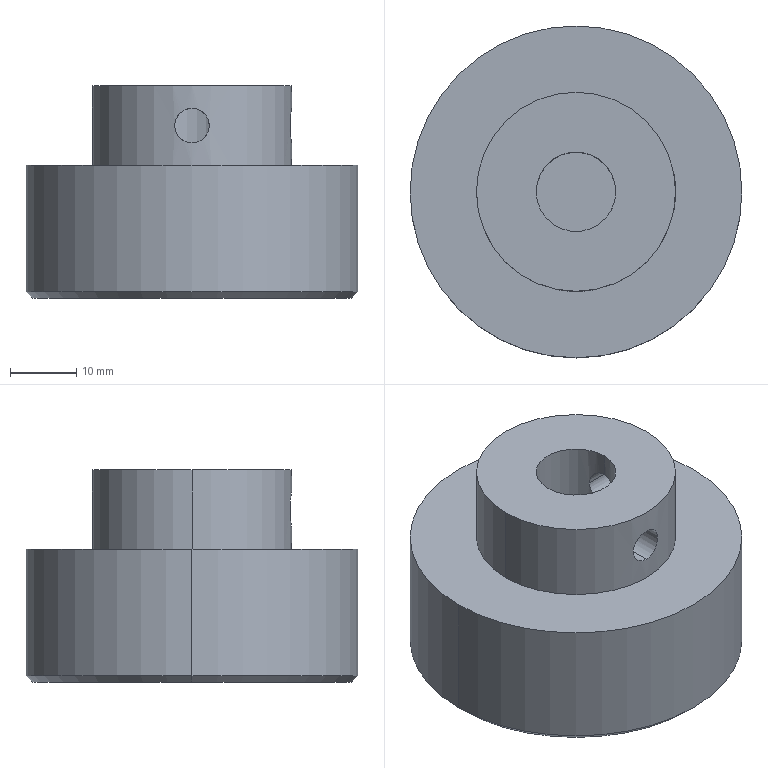Part | STEP file | 1 solid | 16 faces | box 50 x 50 x 32 mm | volume 44461 mm3 | cylinder 10 | plane 4 | cone 2 | commonest cylinder face diameters 5.2 x4 12 x2 30 x2 50 x2